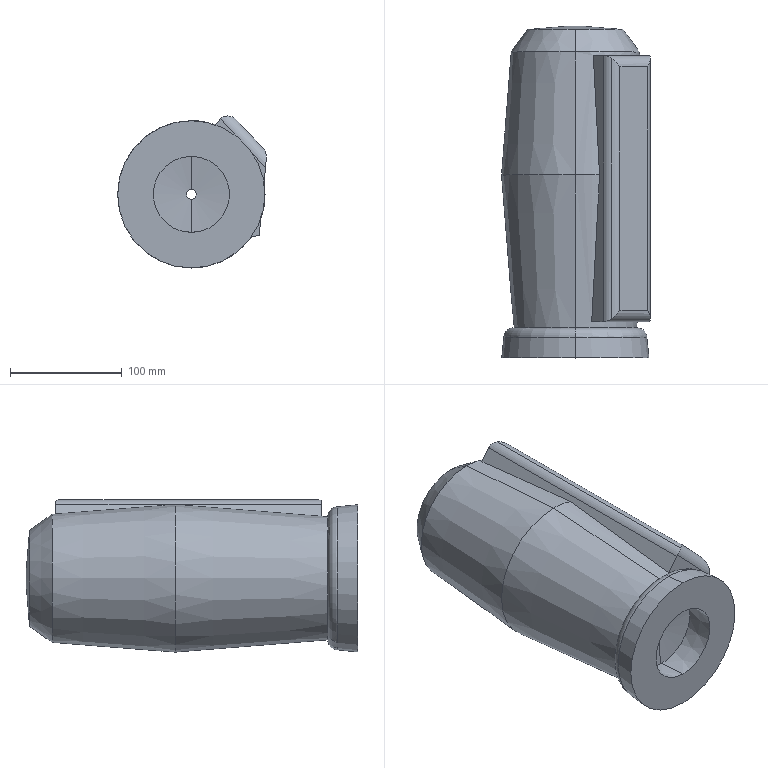Part | SolidWorks | features Revolution 2, Fillet 1, ICE 1 | 2 solids | 44 faces | box 133.247 x 297.006 x 136.186 mm | volume 3477471 mm3 | cone 22 | plane 11 | cylinder 5 | torus 4 | spline 2 | commonest cylinder face diameters 20 x5